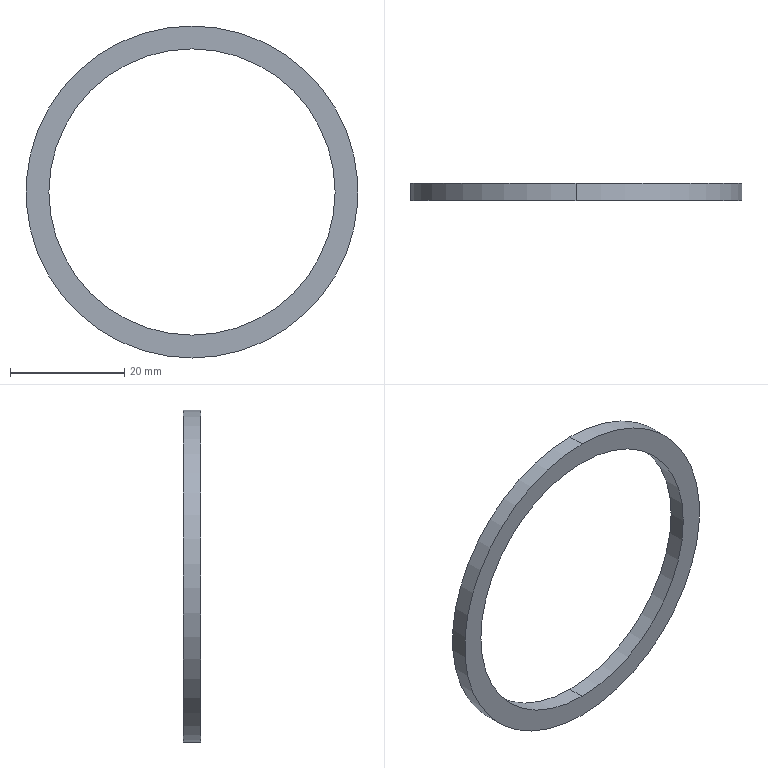Part | SolidWorks | features Extrusion 1 | 1 solid | 6 faces | box 58 x 3 x 58 mm | volume 2036 mm3 | cylinder 4 | plane 2 | commonest cylinder face diameters 50 x2 58 x2
STEP:
#1=CARTESIAN_POINT('',(0.,3.,-25.));
#2=VERTEX_POINT('',#1);
#3=CARTESIAN_POINT('',(0.,3.,25.));
#4=VERTEX_POINT('',#3);
#5=CARTESIAN_POINT('',(0.,3.,0.));
#6=DIRECTION('',(0.,1.,0.));
#7=DIRECTION('',(0.,0.,1.));
#8=AXIS2_PLACEMENT_3D('',#5,#6,#7);
#9=CIRCLE('',#8,25.);
#10=EDGE_CURVE('',#2,#4,#9,.T.);
#11=ORIENTED_EDGE('',*,*,#10,.T.);
#12=CARTESIAN_POINT('',(0.,0.,25.));
#13=VERTEX_POINT('',#12);
#14=CARTESIAN_POINT('',(0.,3.,25.));
#15=DIRECTION('',(0.,-1.,0.));
#16=VECTOR('',#15,1000.);
#17=LINE('',#14,#16);
#18=EDGE_CURVE('',#4,#13,#17,.T.);
#19=ORIENTED_EDGE('',*,*,#18,.T.);
#20=CARTESIAN_POINT('',(0.,0.,-25.));
#21=VERTEX_POINT('',#20);
#22=CARTESIAN_POINT('',(0.,0.,0.));
#23=DIRECTION('',(0.,1.,0.));
#24=DIRECTION('',(0.,0.,1.));
#25=AXIS2_PLACEMENT_3D('',#22,#23,#24);
#26=CIRCLE('',#25,25.);
#27=EDGE_CURVE('',#21,#13,#26,.T.);
#28=ORIENTED_EDGE('',*,*,#27,.F.);
#29=CARTESIAN_POINT('',(0.,3.,-25.));
#30=DIRECTION('',(0.,-1.,0.));
#31=VECTOR('',#30,1000.);
#32=LINE('',#29,#31);
#33=EDGE_CURVE('',#2,#21,#32,.T.);
#34=ORIENTED_EDGE('',*,*,#33,.F.);
#35=EDGE_LOOP('',(#11,#19,#28,#34));
#36=FACE_OUTER_BOUND('',#35,.T.);
#37=CARTESIAN_POINT('',(0.,3.,0.));
#38=DIRECTION('',(0.,-1.,0.));
#39=DIRECTION('',(0.,0.,-1.));
#40=AXIS2_PLACEMENT_3D('',#37,#38,#39);
#41=CYLINDRICAL_SURFACE('',#40,25.);
#42=ADVANCED_FACE('',(#36),#41,.F.);
#43=CARTESIAN_POINT('',(0.,3.,29.));
#44=VERTEX_POINT('',#43);
#45=CARTESIAN_POINT('',(0.,3.,-29.));
#46=VERTEX_POINT('',#45);
#47=CARTESIAN_POINT('',(0.,3.,0.));
#48=DIRECTION('',(0.,1.,0.));
#49=DIRECTION('',(0.,0.,1.));
#50=AXIS2_PLACEMENT_3D('',#47,#48,#49);
#51=CIRCLE('',#50,29.);
#52=EDGE_CURVE('',#44,#46,#51,.T.);
#53=ORIENTED_EDGE('',*,*,#52,.F.);
#54=CARTESIAN_POINT('',(0.,0.,29.));
#55=VERTEX_POINT('',#54);
#56=CARTESIAN_POINT('',(0.,3.,29.));
#57=DIRECTION('',(0.,-1.,0.));
#58=VECTOR('',#57,1000.);
#59=LINE('',#56,#58);
#60=EDGE_CURVE('',#44,#55,#59,.T.);
#61=ORIENTED_EDGE('',*,*,#60,.T.);
#62=CARTESIAN_POINT('',(0.,0.,-29.));
#63=VERTEX_POINT('',#62);
#64=CARTESIAN_POINT('',(0.,0.,0.));
#65=DIRECTION('',(0.,1.,0.));
#66=DIRECTION('',(0.,0.,1.));
#67=AXIS2_PLACEMENT_3D('',#64,#65,#66);
#68=CIRCLE('',#67,29.);
#69=EDGE_CURVE('',#55,#63,#68,.T.);
#70=ORIENTED_EDGE('',*,*,#69,.T.);
#71=CARTESIAN_POINT('',(0.,3.,-29.));
#72=DIRECTION('',(0.,-1.,0.));
#73=VECTOR('',#72,1000.);
#74=LINE('',#71,#73);
#75=EDGE_CURVE('',#46,#63,#74,.T.);
#76=ORIENTED_EDGE('',*,*,#75,.F.);
#77=EDGE_LOOP('',(#53,#61,#70,#76));
#78=FACE_OUTER_BOUND('',#77,.T.);
#79=CARTESIAN_POINT('',(0.,3.,0.));
#80=DIRECTION('',(0.,-1.,0.));
#81=DIRECTION('',(0.,0.,-1.));
#82=AXIS2_PLACEMENT_3D('',#79,#80,#81);
#83=CYLINDRICAL_SURFACE('',#82,29.);
#84=ADVANCED_FACE('',(#78),#83,.T.);
#85=CARTESIAN_POINT('',(0.,3.,0.));
#86=DIRECTION('',(0.,1.,0.));
#87=DIRECTION('',(0.,0.,1.));
#88=AXIS2_PLACEMENT_3D('',#85,#86,#87);
#89=CIRCLE('',#88,29.);
#90=EDGE_CURVE('',#46,#44,#89,.T.);
#91=ORIENTED_EDGE('',*,*,#90,.T.);
#92=ORIENTED_EDGE('',*,*,#52,.T.);
#93=EDGE_LOOP('',(#91,#92));
#94=FACE_OUTER_BOUND('',#93,.T.);
#95=ORIENTED_EDGE('',*,*,#10,.F.);
#96=CARTESIAN_POINT('',(0.,3.,0.));
#97=DIRECTION('',(0.,1.,0.));
#98=DIRECTION('',(0.,0.,1.));
#99=AXIS2_PLACEMENT_3D('',#96,#97,#98);
#100=CIRCLE('',#99,25.);
#101=EDGE_CURVE('',#4,#2,#100,.T.);
#102=ORIENTED_EDGE('',*,*,#101,.F.);
#103=EDGE_LOOP('',(#95,#102));
#104=FACE_BOUND('',#103,.T.);
#105=CARTESIAN_POINT('',(0.,3.,0.));
#106=DIRECTION('',(0.,1.,0.));
#107=DIRECTION('',(0.,0.,1.));
#108=AXIS2_PLACEMENT_3D('',#105,#106,#107);
#109=PLANE('',#108);
#110=ADVANCED_FACE('',(#94,#104),#109,.T.);
#111=CARTESIAN_POINT('',(0.,0.,0.));
#112=DIRECTION('',(0.,1.,0.));
#113=DIRECTION('',(0.,0.,1.));
#114=AXIS2_PLACEMENT_3D('',#111,#112,#113);
#115=CIRCLE('',#114,29.);
#116=EDGE_CURVE('',#63,#55,#115,.T.);
#117=ORIENTED_EDGE('',*,*,#116,.F.);
#118=ORIENTED_EDGE('',*,*,#69,.F.);
#119=EDGE_LOOP('',(#117,#118));
#120=FACE_OUTER_BOUND('',#119,.T.);
#121=ORIENTED_EDGE('',*,*,#27,.T.);
#122=CARTESIAN_POINT('',(0.,0.,0.));
#123=DIRECTION('',(0.,1.,0.));
#124=DIRECTION('',(0.,0.,1.));
#125=AXIS2_PLACEMENT_3D('',#122,#123,#124);
#126=CIRCLE('',#125,25.);
#127=EDGE_CURVE('',#13,#21,#126,.T.);
#128=ORIENTED_EDGE('',*,*,#127,.T.);
#129=EDGE_LOOP('',(#121,#128));
#130=FACE_BOUND('',#129,.T.);
#131=CARTESIAN_POINT('',(0.,0.,0.));
#132=DIRECTION('',(0.,1.,0.));
#133=DIRECTION('',(0.,0.,1.));
#134=AXIS2_PLACEMENT_3D('',#131,#132,#133);
#135=PLANE('',#134);
#136=ADVANCED_FACE('',(#120,#130),#135,.F.);
#137=ORIENTED_EDGE('',*,*,#60,.F.);
#138=ORIENTED_EDGE('',*,*,#90,.F.);
#139=ORIENTED_EDGE('',*,*,#75,.T.);
#140=ORIENTED_EDGE('',*,*,#116,.T.);
#141=EDGE_LOOP('',(#137,#138,#139,#140));
#142=FACE_OUTER_BOUND('',#141,.T.);
#143=CARTESIAN_POINT('',(0.,3.,0.));
#144=DIRECTION('',(0.,-1.,0.));
#145=DIRECTION('',(0.,0.,-1.));
#146=AXIS2_PLACEMENT_3D('',#143,#144,#145);
#147=CYLINDRICAL_SURFACE('',#146,29.);
#148=ADVANCED_FACE('',(#142),#147,.T.);
#149=ORIENTED_EDGE('',*,*,#18,.F.);
#150=ORIENTED_EDGE('',*,*,#101,.T.);
#151=ORIENTED_EDGE('',*,*,#33,.T.);
#152=ORIENTED_EDGE('',*,*,#127,.F.);
#153=EDGE_LOOP('',(#149,#150,#151,#152));
#154=FACE_OUTER_BOUND('',#153,.T.);
#155=CARTESIAN_POINT('',(0.,3.,0.));
#156=DIRECTION('',(0.,-1.,0.));
#157=DIRECTION('',(0.,0.,-1.));
#158=AXIS2_PLACEMENT_3D('',#155,#156,#157);
#159=CYLINDRICAL_SURFACE('',#158,25.);
#160=ADVANCED_FACE('',(#154),#159,.F.);
#161=CLOSED_SHELL('',(#42,#84,#110,#136,#148,#160));
#162=MANIFOLD_SOLID_BREP('',#161);
#163=CARTESIAN_POINT('',(0.,0.,0.));
#164=DIRECTION('',(0.,0.,1.));
#165=DIRECTION('',(1.,0.,0.));
#166=AXIS2_PLACEMENT_3D('',#163,#164,#165);
#167=(LENGTH_UNIT()NAMED_UNIT(*)SI_UNIT(.MILLI.,.METRE.));
#168=UNCERTAINTY_MEASURE_WITH_UNIT(LENGTH_MEASURE(0.00001),#167,'','');
#169=(NAMED_UNIT(*)PLANE_ANGLE_UNIT()SI_UNIT($,.RADIAN.));
#170=(NAMED_UNIT(*)SI_UNIT($,.STERADIAN.)SOLID_ANGLE_UNIT());
#171=(GEOMETRIC_REPRESENTATION_CONTEXT(3)GLOBAL_UNCERTAINTY_ASSIGNED_CONTEXT((#168))GLOBAL_UNIT_ASSIGNED_CONTEXT((#167,#169,#170))REPRESENTATION_CONTEXT('',''));
#172=ADVANCED_BREP_SHAPE_REPRESENTATION('',(#162,#166),#171);